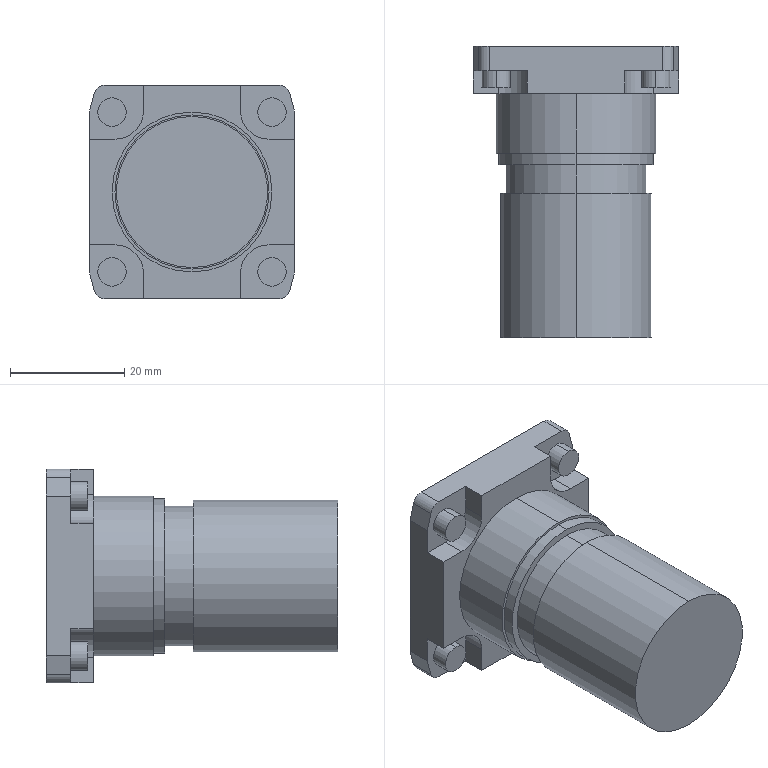Part | STEP file | AR-20_BONNET_HI | 1 solid | 54 faces | box 36 x 51.1 x 37.5 mm | volume 33945 mm3 | plane 30 | cylinder 24 | commonest cylinder face diameters 5 x8 4 x4 10 x4 24.5 x2 26.5 x2 27 x2